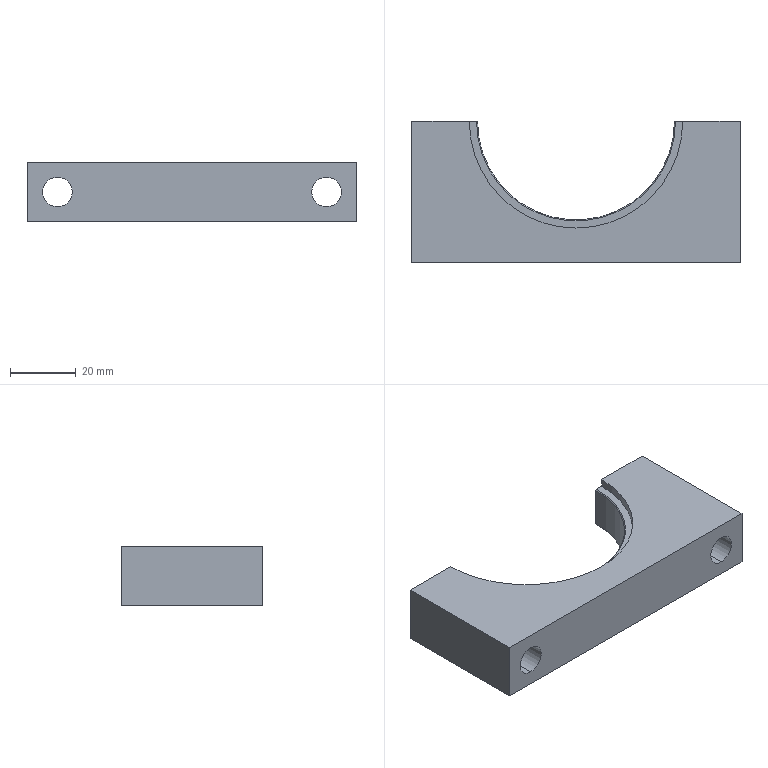Part | SolidWorks | features HoleWzd 2, ICE 2, Chamfer 1, Extrusion 1 | 1 solid | 21 faces | box 100 x 43 x 18 mm | volume 45196 mm3 | plane 10 | cylinder 9 | cone 2 | commonest cylinder face diameters 9 x4 4 x2 65 x2 60 x1
STEP:
#1=CARTESIAN_POINT('',(0.,-34.,7.));
#2=VERTEX_POINT('',#1);
#3=CARTESIAN_POINT('',(0.,-34.,11.));
#4=VERTEX_POINT('',#3);
#5=CARTESIAN_POINT('',(0.,-34.,9.));
#6=DIRECTION('',(0.,1.,0.));
#7=DIRECTION('',(0.,0.,1.));
#8=AXIS2_PLACEMENT_3D('',#5,#6,#7);
#9=CIRCLE('',#8,2.);
#10=EDGE_CURVE('',#2,#4,#9,.T.);
#11=ORIENTED_EDGE('',*,*,#10,.F.);
#12=CARTESIAN_POINT('',(0.,-30.,7.));
#13=VERTEX_POINT('',#12);
#14=CARTESIAN_POINT('',(0.,0.,7.));
#15=DIRECTION('',(0.,1.,0.));
#16=VECTOR('',#15,1000.);
#17=LINE('',#14,#16);
#18=EDGE_CURVE('',#2,#13,#17,.T.);
#19=ORIENTED_EDGE('',*,*,#18,.T.);
#20=CARTESIAN_POINT('',(0.,-30.,11.));
#21=VERTEX_POINT('',#20);
#22=CARTESIAN_POINT('',(0.,-30.,11.));
#23=CARTESIAN_POINT('',(-0.1322,-30.,11.));
#24=CARTESIAN_POINT('',(-0.2622,-29.999,10.987));
#25=CARTESIAN_POINT('',(-0.5178,-29.996,10.936));
#26=CARTESIAN_POINT('',(-0.6449,-29.993,10.898));
#27=CARTESIAN_POINT('',(-0.8871,-29.987,10.797));
#28=CARTESIAN_POINT('',(-1.002,-29.983,10.736));
#29=CARTESIAN_POINT('',(-1.219,-29.975,10.591));
#30=CARTESIAN_POINT('',(-1.322,-29.971,10.506));
#31=CARTESIAN_POINT('',(-1.599,-29.958,10.229));
#32=CARTESIAN_POINT('',(-1.748,-29.949,10.006));
#33=CARTESIAN_POINT('',(-1.947,-29.937,9.525));
#34=CARTESIAN_POINT('',(-2.,-29.933,9.262));
#35=CARTESIAN_POINT('',(-2.,-29.933,8.87));
#36=CARTESIAN_POINT('',(-1.987,-29.934,8.738));
#37=CARTESIAN_POINT('',(-1.936,-29.937,8.481));
#38=CARTESIAN_POINT('',(-1.898,-29.94,8.356));
#39=CARTESIAN_POINT('',(-1.798,-29.946,8.114));
#40=CARTESIAN_POINT('',(-1.735,-29.95,7.997));
#41=CARTESIAN_POINT('',(-1.591,-29.958,7.78));
#42=CARTESIAN_POINT('',(-1.508,-29.962,7.679));
#43=CARTESIAN_POINT('',(-1.321,-29.971,7.493));
#44=CARTESIAN_POINT('',(-1.22,-29.975,7.41));
#45=CARTESIAN_POINT('',(-1.003,-29.983,7.265));
#46=CARTESIAN_POINT('',(-0.8865,-29.987,7.202));
#47=CARTESIAN_POINT('',(-0.6442,-29.993,7.102));
#48=CARTESIAN_POINT('',(-0.5195,-29.996,7.064));
#49=CARTESIAN_POINT('',(-0.2631,-29.999,7.013));
#50=CARTESIAN_POINT('',(-0.1305,-30.,7.));
#51=CARTESIAN_POINT('',(0.,-30.,7.));
#52=B_SPLINE_CURVE_WITH_KNOTS('',3,(#22,#23,#24,#25,#26,#27,#28,#29,#30,#31,#32,#33,#34,#35,#36,#37,#38,#39,#40,#41,#42,#43,#44,#45,#46,#47,#48,#49,#50,#51),.UNSPECIFIED.,.F.,.F.,(4,2,2,2,2,2,2,2,2,2,2,2,2,2,4),(0.,0.0003909,0.0007818,0.001173,0.001564,0.002345,0.003127,0.003518,0.003909,0.0043,0.004691,0.005082,0.005473,0.005864,0.006255),.UNSPECIFIED.);
#53=EDGE_CURVE('',#21,#13,#52,.T.);
#54=ORIENTED_EDGE('',*,*,#53,.F.);
#55=CARTESIAN_POINT('',(0.,0.,11.));
#56=DIRECTION('',(0.,1.,0.));
#57=VECTOR('',#56,1000.);
#58=LINE('',#55,#57);
#59=EDGE_CURVE('',#4,#21,#58,.T.);
#60=ORIENTED_EDGE('',*,*,#59,.F.);
#61=EDGE_LOOP('',(#11,#19,#54,#60));
#62=FACE_OUTER_BOUND('',#61,.T.);
#63=CARTESIAN_POINT('',(0.,0.,9.));
#64=DIRECTION('',(0.,1.,0.));
#65=DIRECTION('',(0.,0.,1.));
#66=AXIS2_PLACEMENT_3D('',#63,#64,#65);
#67=CYLINDRICAL_SURFACE('',#66,2.);
#68=ADVANCED_FACE('',(#62),#67,.F.);
#69=CARTESIAN_POINT('',(-41.,-43.,4.5));
#70=VERTEX_POINT('',#69);
#71=CARTESIAN_POINT('',(-41.,-43.,13.5));
#72=VERTEX_POINT('',#71);
#73=CARTESIAN_POINT('',(-41.,-43.,9.));
#74=DIRECTION('',(0.,1.,0.));
#75=DIRECTION('',(0.,0.,1.));
#76=AXIS2_PLACEMENT_3D('',#73,#74,#75);
#77=CIRCLE('',#76,4.5);
#78=EDGE_CURVE('',#70,#72,#77,.T.);
#79=ORIENTED_EDGE('',*,*,#78,.F.);
#80=CARTESIAN_POINT('',(-41.,0.,4.5));
#81=VERTEX_POINT('',#80);
#82=CARTESIAN_POINT('',(-41.,0.,4.5));
#83=DIRECTION('',(0.,1.,0.));
#84=VECTOR('',#83,1000.);
#85=LINE('',#82,#84);
#86=EDGE_CURVE('',#70,#81,#85,.T.);
#87=ORIENTED_EDGE('',*,*,#86,.T.);
#88=CARTESIAN_POINT('',(-41.,0.,13.5));
#89=VERTEX_POINT('',#88);
#90=CARTESIAN_POINT('',(-41.,0.,9.));
#91=DIRECTION('',(0.,1.,0.));
#92=DIRECTION('',(0.,0.,1.));
#93=AXIS2_PLACEMENT_3D('',#90,#91,#92);
#94=CIRCLE('',#93,4.5);
#95=EDGE_CURVE('',#81,#89,#94,.T.);
#96=ORIENTED_EDGE('',*,*,#95,.T.);
#97=CARTESIAN_POINT('',(-41.,0.,13.5));
#98=DIRECTION('',(0.,1.,0.));
#99=VECTOR('',#98,1000.);
#100=LINE('',#97,#99);
#101=EDGE_CURVE('',#72,#89,#100,.T.);
#102=ORIENTED_EDGE('',*,*,#101,.F.);
#103=EDGE_LOOP('',(#79,#87,#96,#102));
#104=FACE_OUTER_BOUND('',#103,.T.);
#105=CARTESIAN_POINT('',(-41.,0.,9.));
#106=DIRECTION('',(0.,1.,0.));
#107=DIRECTION('',(0.,0.,1.));
#108=AXIS2_PLACEMENT_3D('',#105,#106,#107);
#109=CYLINDRICAL_SURFACE('',#108,4.5);
#110=ADVANCED_FACE('',(#104),#109,.F.);
#111=CARTESIAN_POINT('',(41.,-43.,4.5));
#112=VERTEX_POINT('',#111);
#113=CARTESIAN_POINT('',(41.,-43.,13.5));
#114=VERTEX_POINT('',#113);
#115=CARTESIAN_POINT('',(41.,-43.,9.));
#116=DIRECTION('',(0.,1.,0.));
#117=DIRECTION('',(0.,0.,1.));
#118=AXIS2_PLACEMENT_3D('',#115,#116,#117);
#119=CIRCLE('',#118,4.5);
#120=EDGE_CURVE('',#112,#114,#119,.T.);
#121=ORIENTED_EDGE('',*,*,#120,.F.);
#122=CARTESIAN_POINT('',(41.,0.,4.5));
#123=VERTEX_POINT('',#122);
#124=CARTESIAN_POINT('',(41.,0.,4.5));
#125=DIRECTION('',(0.,1.,0.));
#126=VECTOR('',#125,1000.);
#127=LINE('',#124,#126);
#128=EDGE_CURVE('',#112,#123,#127,.T.);
#129=ORIENTED_EDGE('',*,*,#128,.T.);
#130=CARTESIAN_POINT('',(41.,0.,13.5));
#131=VERTEX_POINT('',#130);
#132=CARTESIAN_POINT('',(41.,0.,9.));
#133=DIRECTION('',(0.,1.,0.));
#134=DIRECTION('',(0.,0.,1.));
#135=AXIS2_PLACEMENT_3D('',#132,#133,#134);
#136=CIRCLE('',#135,4.5);
#137=EDGE_CURVE('',#123,#131,#136,.T.);
#138=ORIENTED_EDGE('',*,*,#137,.T.);
#139=CARTESIAN_POINT('',(41.,0.,13.5));
#140=DIRECTION('',(0.,1.,0.));
#141=VECTOR('',#140,1000.);
#142=LINE('',#139,#141);
#143=EDGE_CURVE('',#114,#131,#142,.T.);
#144=ORIENTED_EDGE('',*,*,#143,.F.);
#145=EDGE_LOOP('',(#121,#129,#138,#144));
#146=FACE_OUTER_BOUND('',#145,.T.);
#147=CARTESIAN_POINT('',(41.,0.,9.));
#148=DIRECTION('',(0.,1.,0.));
#149=DIRECTION('',(0.,0.,1.));
#150=AXIS2_PLACEMENT_3D('',#147,#148,#149);
#151=CYLINDRICAL_SURFACE('',#150,4.5);
#152=ADVANCED_FACE('',(#146),#151,.F.);
#153=ORIENTED_EDGE('',*,*,#53,.T.);
#154=CARTESIAN_POINT('',(0.,-30.,7.));
#155=CARTESIAN_POINT('',(0.261,-30.,7.));
#156=CARTESIAN_POINT('',(0.5242,-29.996,7.052));
#157=CARTESIAN_POINT('',(1.006,-29.984,7.252));
#158=CARTESIAN_POINT('',(1.229,-29.975,7.401));
#159=CARTESIAN_POINT('',(1.505,-29.962,7.677));
#160=CARTESIAN_POINT('',(1.59,-29.958,7.78));
#161=CARTESIAN_POINT('',(1.735,-29.95,7.997));
#162=CARTESIAN_POINT('',(1.797,-29.946,8.112));
#163=CARTESIAN_POINT('',(1.897,-29.94,8.354));
#164=CARTESIAN_POINT('',(1.936,-29.937,8.481));
#165=CARTESIAN_POINT('',(1.987,-29.934,8.737));
#166=CARTESIAN_POINT('',(2.,-29.933,8.866));
#167=CARTESIAN_POINT('',(2.,-29.933,9.13));
#168=CARTESIAN_POINT('',(1.987,-29.934,9.261));
#169=CARTESIAN_POINT('',(1.937,-29.937,9.516));
#170=CARTESIAN_POINT('',(1.898,-29.94,9.643));
#171=CARTESIAN_POINT('',(1.798,-29.946,9.886));
#172=CARTESIAN_POINT('',(1.737,-29.95,10.001));
#173=CARTESIAN_POINT('',(1.592,-29.958,10.218));
#174=CARTESIAN_POINT('',(1.507,-29.962,10.321));
#175=CARTESIAN_POINT('',(1.323,-29.971,10.506));
#176=CARTESIAN_POINT('',(1.222,-29.975,10.588));
#177=CARTESIAN_POINT('',(1.004,-29.983,10.735));
#178=CARTESIAN_POINT('',(0.8877,-29.987,10.797));
#179=CARTESIAN_POINT('',(0.5269,-29.996,10.947));
#180=CARTESIAN_POINT('',(0.2643,-30.,11.));
#181=CARTESIAN_POINT('',(0.,-30.,11.));
#182=B_SPLINE_CURVE_WITH_KNOTS('',3,(#154,#155,#156,#157,#158,#159,#160,#161,#162,#163,#164,#165,#166,#167,#168,#169,#170,#171,#172,#173,#174,#175,#176,#177,#178,#179,#180,#181),.UNSPECIFIED.,.F.,.F.,(4,2,2,2,2,2,2,2,2,2,2,2,2,4),(0.006255,0.007036,0.007818,0.008209,0.0086,0.00899,0.009381,0.009772,0.01016,0.01055,0.01094,0.01134,0.01173,0.01251),.UNSPECIFIED.);
#183=EDGE_CURVE('',#13,#21,#182,.T.);
#184=ORIENTED_EDGE('',*,*,#183,.T.);
#185=EDGE_LOOP('',(#153,#184));
#186=FACE_BOUND('',#185,.T.);
#187=CARTESIAN_POINT('',(30.,0.,15.2));
#188=VERTEX_POINT('',#187);
#189=CARTESIAN_POINT('',(30.,0.,2.8));
#190=VERTEX_POINT('',#189);
#191=CARTESIAN_POINT('',(30.,0.,18.));
#192=DIRECTION('',(0.,0.,-1.));
#193=VECTOR('',#192,1000.);
#194=LINE('',#191,#193);
#195=EDGE_CURVE('',#188,#190,#194,.T.);
#196=ORIENTED_EDGE('',*,*,#195,.T.);
#197=CARTESIAN_POINT('',(-30.,0.,2.8));
#198=VERTEX_POINT('',#197);
#199=CARTESIAN_POINT('',(0.,0.,2.8));
#200=DIRECTION('',(0.,0.,-1.));
#201=DIRECTION('',(-1.,0.,0.));
#202=AXIS2_PLACEMENT_3D('',#199,#200,#201);
#203=CIRCLE('',#202,30.);
#204=EDGE_CURVE('',#190,#198,#203,.T.);
#205=ORIENTED_EDGE('',*,*,#204,.T.);
#206=CARTESIAN_POINT('',(-30.,0.,15.2));
#207=VERTEX_POINT('',#206);
#208=CARTESIAN_POINT('',(-30.,0.,18.));
#209=DIRECTION('',(0.,0.,-1.));
#210=VECTOR('',#209,1000.);
#211=LINE('',#208,#210);
#212=EDGE_CURVE('',#207,#198,#211,.T.);
#213=ORIENTED_EDGE('',*,*,#212,.F.);
#214=CARTESIAN_POINT('',(0.,0.,15.2));
#215=DIRECTION('',(0.,0.,1.));
#216=DIRECTION('',(1.,0.,0.));
#217=AXIS2_PLACEMENT_3D('',#214,#215,#216);
#218=CIRCLE('',#217,30.);
#219=EDGE_CURVE('',#207,#188,#218,.T.);
#220=ORIENTED_EDGE('',*,*,#219,.T.);
#221=EDGE_LOOP('',(#196,#205,#213,#220));
#222=FACE_OUTER_BOUND('',#221,.T.);
#223=CARTESIAN_POINT('',(0.,0.,18.));
#224=DIRECTION('',(0.,0.,-1.));
#225=DIRECTION('',(-1.,0.,0.));
#226=AXIS2_PLACEMENT_3D('',#223,#224,#225);
#227=CYLINDRICAL_SURFACE('',#226,30.);
#228=ADVANCED_FACE('',(#186,#222),#227,.F.);
#229=CARTESIAN_POINT('',(-41.,0.,9.));
#230=DIRECTION('',(0.,1.,0.));
#231=DIRECTION('',(0.,0.,1.));
#232=AXIS2_PLACEMENT_3D('',#229,#230,#231);
#233=CIRCLE('',#232,4.5);
#234=EDGE_CURVE('',#89,#81,#233,.T.);
#235=ORIENTED_EDGE('',*,*,#234,.F.);
#236=ORIENTED_EDGE('',*,*,#95,.F.);
#237=EDGE_LOOP('',(#235,#236));
#238=FACE_BOUND('',#237,.T.);
#239=ORIENTED_EDGE('',*,*,#212,.T.);
#240=CARTESIAN_POINT('',(-30.3,0.,2.5));
#241=VERTEX_POINT('',#240);
#242=CARTESIAN_POINT('',(0.,0.,32.8));
#243=DIRECTION('',(-0.7071,0.,-0.7071));
#244=VECTOR('',#243,1000.);
#245=LINE('',#242,#244);
#246=EDGE_CURVE('',#198,#241,#245,.T.);
#247=ORIENTED_EDGE('',*,*,#246,.T.);
#248=CARTESIAN_POINT('',(-32.5,0.,2.5));
#249=VERTEX_POINT('',#248);
#250=CARTESIAN_POINT('',(-50.,0.,2.5));
#251=DIRECTION('',(1.,0.,0.));
#252=VECTOR('',#251,1000.);
#253=LINE('',#250,#252);
#254=EDGE_CURVE('',#249,#241,#253,.T.);
#255=ORIENTED_EDGE('',*,*,#254,.F.);
#256=CARTESIAN_POINT('',(-32.5,0.,0.));
#257=VERTEX_POINT('',#256);
#258=CARTESIAN_POINT('',(-32.5,0.,2.5));
#259=DIRECTION('',(0.,0.,-1.));
#260=VECTOR('',#259,1000.);
#261=LINE('',#258,#260);
#262=EDGE_CURVE('',#249,#257,#261,.T.);
#263=ORIENTED_EDGE('',*,*,#262,.T.);
#264=CARTESIAN_POINT('',(-50.,0.,0.));
#265=VERTEX_POINT('',#264);
#266=CARTESIAN_POINT('',(-50.,0.,0.));
#267=DIRECTION('',(-1.,0.,0.));
#268=VECTOR('',#267,1000.);
#269=LINE('',#266,#268);
#270=EDGE_CURVE('',#257,#265,#269,.T.);
#271=ORIENTED_EDGE('',*,*,#270,.T.);
#272=CARTESIAN_POINT('',(-50.,0.,18.));
#273=VERTEX_POINT('',#272);
#274=CARTESIAN_POINT('',(-50.,0.,18.));
#275=DIRECTION('',(0.,0.,-1.));
#276=VECTOR('',#275,1000.);
#277=LINE('',#274,#276);
#278=EDGE_CURVE('',#273,#265,#277,.T.);
#279=ORIENTED_EDGE('',*,*,#278,.F.);
#280=CARTESIAN_POINT('',(-32.5,0.,18.));
#281=VERTEX_POINT('',#280);
#282=CARTESIAN_POINT('',(-50.,0.,18.));
#283=DIRECTION('',(-1.,0.,0.));
#284=VECTOR('',#283,1000.);
#285=LINE('',#282,#284);
#286=EDGE_CURVE('',#281,#273,#285,.T.);
#287=ORIENTED_EDGE('',*,*,#286,.F.);
#288=CARTESIAN_POINT('',(-32.5,0.,15.5));
#289=VERTEX_POINT('',#288);
#290=CARTESIAN_POINT('',(-32.5,0.,15.5));
#291=DIRECTION('',(0.,0.,-1.));
#292=VECTOR('',#291,1000.);
#293=LINE('',#290,#292);
#294=EDGE_CURVE('',#281,#289,#293,.T.);
#295=ORIENTED_EDGE('',*,*,#294,.T.);
#296=CARTESIAN_POINT('',(-30.3,0.,15.5));
#297=VERTEX_POINT('',#296);
#298=CARTESIAN_POINT('',(-50.,0.,15.5));
#299=DIRECTION('',(-1.,0.,0.));
#300=VECTOR('',#299,1000.);
#301=LINE('',#298,#300);
#302=EDGE_CURVE('',#297,#289,#301,.T.);
#303=ORIENTED_EDGE('',*,*,#302,.F.);
#304=CARTESIAN_POINT('',(0.,0.,-14.8));
#305=DIRECTION('',(0.7071,0.,-0.7071));
#306=VECTOR('',#305,1000.);
#307=LINE('',#304,#306);
#308=EDGE_CURVE('',#297,#207,#307,.T.);
#309=ORIENTED_EDGE('',*,*,#308,.T.);
#310=EDGE_LOOP('',(#239,#247,#255,#263,#271,#279,#287,#295,#303,#309));
#311=FACE_OUTER_BOUND('',#310,.T.);
#312=CARTESIAN_POINT('',(-50.,0.,18.));
#313=DIRECTION('',(0.,-1.,0.));
#314=DIRECTION('',(1.,0.,0.));
#315=AXIS2_PLACEMENT_3D('',#312,#313,#314);
#316=PLANE('',#315);
#317=ADVANCED_FACE('',(#238,#311),#316,.F.);
#318=CARTESIAN_POINT('',(-50.,-43.,0.));
#319=VERTEX_POINT('',#318);
#320=CARTESIAN_POINT('',(-50.,-43.,0.));
#321=DIRECTION('',(0.,-1.,0.));
#322=VECTOR('',#321,1000.);
#323=LINE('',#320,#322);
#324=EDGE_CURVE('',#265,#319,#323,.T.);
#325=ORIENTED_EDGE('',*,*,#324,.T.);
#326=CARTESIAN_POINT('',(-50.,-43.,18.));
#327=VERTEX_POINT('',#326);
#328=CARTESIAN_POINT('',(-50.,-43.,18.));
#329=DIRECTION('',(0.,0.,-1.));
#330=VECTOR('',#329,1000.);
#331=LINE('',#328,#330);
#332=EDGE_CURVE('',#327,#319,#331,.T.);
#333=ORIENTED_EDGE('',*,*,#332,.F.);
#334=CARTESIAN_POINT('',(-50.,-43.,18.));
#335=DIRECTION('',(0.,-1.,0.));
#336=VECTOR('',#335,1000.);
#337=LINE('',#334,#336);
#338=EDGE_CURVE('',#273,#327,#337,.T.);
#339=ORIENTED_EDGE('',*,*,#338,.F.);
#340=ORIENTED_EDGE('',*,*,#278,.T.);
#341=EDGE_LOOP('',(#325,#333,#339,#340));
#342=FACE_OUTER_BOUND('',#341,.T.);
#343=CARTESIAN_POINT('',(-50.,-43.,18.));
#344=DIRECTION('',(1.,0.,0.));
#345=DIRECTION('',(0.,0.,-1.));
#346=AXIS2_PLACEMENT_3D('',#343,#344,#345);
#347=PLANE('',#346);
#348=ADVANCED_FACE('',(#342),#347,.F.);
#349=CARTESIAN_POINT('',(-41.,-43.,9.));
#350=DIRECTION('',(0.,1.,0.));
#351=DIRECTION('',(0.,0.,1.));
#352=AXIS2_PLACEMENT_3D('',#349,#350,#351);
#353=CIRCLE('',#352,4.5);
#354=EDGE_CURVE('',#72,#70,#353,.T.);
#355=ORIENTED_EDGE('',*,*,#354,.T.);
#356=ORIENTED_EDGE('',*,*,#78,.T.);
#357=EDGE_LOOP('',(#355,#356));
#358=FACE_BOUND('',#357,.T.);
#359=CARTESIAN_POINT('',(41.,-43.,9.));
#360=DIRECTION('',(0.,1.,0.));
#361=DIRECTION('',(0.,0.,1.));
#362=AXIS2_PLACEMENT_3D('',#359,#360,#361);
#363=CIRCLE('',#362,4.5);
#364=EDGE_CURVE('',#114,#112,#363,.T.);
#365=ORIENTED_EDGE('',*,*,#364,.T.);
#366=ORIENTED_EDGE('',*,*,#120,.T.);
#367=EDGE_LOOP('',(#365,#366));
#368=FACE_BOUND('',#367,.T.);
#369=CARTESIAN_POINT('',(50.,-43.,0.));
#370=VERTEX_POINT('',#369);
#371=CARTESIAN_POINT('',(-50.,-43.,0.));
#372=DIRECTION('',(1.,0.,0.));
#373=VECTOR('',#372,1000.);
#374=LINE('',#371,#373);
#375=EDGE_CURVE('',#319,#370,#374,.T.);
#376=ORIENTED_EDGE('',*,*,#375,.T.);
#377=CARTESIAN_POINT('',(50.,-43.,18.));
#378=VERTEX_POINT('',#377);
#379=CARTESIAN_POINT('',(50.,-43.,18.));
#380=DIRECTION('',(0.,0.,-1.));
#381=VECTOR('',#380,1000.);
#382=LINE('',#379,#381);
#383=EDGE_CURVE('',#378,#370,#382,.T.);
#384=ORIENTED_EDGE('',*,*,#383,.F.);
#385=CARTESIAN_POINT('',(-50.,-43.,18.));
#386=DIRECTION('',(1.,0.,0.));
#387=VECTOR('',#386,1000.);
#388=LINE('',#385,#387);
#389=EDGE_CURVE('',#327,#378,#388,.T.);
#390=ORIENTED_EDGE('',*,*,#389,.F.);
#391=ORIENTED_EDGE('',*,*,#332,.T.);
#392=EDGE_LOOP('',(#376,#384,#390,#391));
#393=FACE_OUTER_BOUND('',#392,.T.);
#394=CARTESIAN_POINT('',(-50.,-43.,18.));
#395=DIRECTION('',(0.,1.,0.));
#396=DIRECTION('',(-1.,0.,0.));
#397=AXIS2_PLACEMENT_3D('',#394,#395,#396);
#398=PLANE('',#397);
#399=ADVANCED_FACE('',(#358,#368,#393),#398,.F.);
#400=CARTESIAN_POINT('',(50.,0.,0.));
#401=VERTEX_POINT('',#400);
#402=CARTESIAN_POINT('',(50.,-43.,0.));
#403=DIRECTION('',(0.,1.,0.));
#404=VECTOR('',#403,1000.);
#405=LINE('',#402,#404);
#406=EDGE_CURVE('',#370,#401,#405,.T.);
#407=ORIENTED_EDGE('',*,*,#406,.T.);
#408=CARTESIAN_POINT('',(50.,0.,18.));
#409=VERTEX_POINT('',#408);
#410=CARTESIAN_POINT('',(50.,0.,18.));
#411=DIRECTION('',(0.,0.,-1.));
#412=VECTOR('',#411,1000.);
#413=LINE('',#410,#412);
#414=EDGE_CURVE('',#409,#401,#413,.T.);
#415=ORIENTED_EDGE('',*,*,#414,.F.);
#416=CARTESIAN_POINT('',(50.,-43.,18.));
#417=DIRECTION('',(0.,1.,0.));
#418=VECTOR('',#417,1000.);
#419=LINE('',#416,#418);
#420=EDGE_CURVE('',#378,#409,#419,.T.);
#421=ORIENTED_EDGE('',*,*,#420,.F.);
#422=ORIENTED_EDGE('',*,*,#383,.T.);
#423=EDGE_LOOP('',(#407,#415,#421,#422));
#424=FACE_OUTER_BOUND('',#423,.T.);
#425=CARTESIAN_POINT('',(50.,-43.,18.));
#426=DIRECTION('',(-1.,0.,0.));
#427=DIRECTION('',(0.,-1.,0.));
#428=AXIS2_PLACEMENT_3D('',#425,#426,#427);
#429=PLANE('',#428);
#430=ADVANCED_FACE('',(#424),#429,.F.);
#431=CARTESIAN_POINT('',(41.,0.,9.));
#432=DIRECTION('',(0.,1.,0.));
#433=DIRECTION('',(0.,0.,1.));
#434=AXIS2_PLACEMENT_3D('',#431,#432,#433);
#435=CIRCLE('',#434,4.5);
#436=EDGE_CURVE('',#131,#123,#435,.T.);
#437=ORIENTED_EDGE('',*,*,#436,.F.);
#438=ORIENTED_EDGE('',*,*,#137,.F.);
#439=EDGE_LOOP('',(#437,#438));
#440=FACE_BOUND('',#439,.T.);
#441=CARTESIAN_POINT('',(30.3,0.,2.5));
#442=VERTEX_POINT('',#441);
#443=CARTESIAN_POINT('',(32.5,0.,2.5));
#444=VERTEX_POINT('',#443);
#445=CARTESIAN_POINT('',(30.,0.,2.5));
#446=DIRECTION('',(1.,0.,0.));
#447=VECTOR('',#446,1000.);
#448=LINE('',#445,#447);
#449=EDGE_CURVE('',#442,#444,#448,.T.);
#450=ORIENTED_EDGE('',*,*,#449,.F.);
#451=CARTESIAN_POINT('',(0.,0.,32.8));
#452=DIRECTION('',(-0.7071,0.,0.7071));
#453=VECTOR('',#452,1000.);
#454=LINE('',#451,#453);
#455=EDGE_CURVE('',#442,#190,#454,.T.);
#456=ORIENTED_EDGE('',*,*,#455,.T.);
#457=ORIENTED_EDGE('',*,*,#195,.F.);
#458=CARTESIAN_POINT('',(30.3,0.,15.5));
#459=VERTEX_POINT('',#458);
#460=CARTESIAN_POINT('',(0.,0.,-14.8));
#461=DIRECTION('',(0.7071,0.,0.7071));
#462=VECTOR('',#461,1000.);
#463=LINE('',#460,#462);
#464=EDGE_CURVE('',#188,#459,#463,.T.);
#465=ORIENTED_EDGE('',*,*,#464,.T.);
#466=CARTESIAN_POINT('',(32.5,0.,15.5));
#467=VERTEX_POINT('',#466);
#468=CARTESIAN_POINT('',(30.,0.,15.5));
#469=DIRECTION('',(-1.,0.,0.));
#470=VECTOR('',#469,1000.);
#471=LINE('',#468,#470);
#472=EDGE_CURVE('',#467,#459,#471,.T.);
#473=ORIENTED_EDGE('',*,*,#472,.F.);
#474=CARTESIAN_POINT('',(32.5,0.,18.));
#475=VERTEX_POINT('',#474);
#476=CARTESIAN_POINT('',(32.5,0.,15.5));
#477=DIRECTION('',(0.,0.,1.));
#478=VECTOR('',#477,1000.);
#479=LINE('',#476,#478);
#480=EDGE_CURVE('',#467,#475,#479,.T.);
#481=ORIENTED_EDGE('',*,*,#480,.T.);
#482=CARTESIAN_POINT('',(30.,0.,18.));
#483=DIRECTION('',(-1.,0.,0.));
#484=VECTOR('',#483,1000.);
#485=LINE('',#482,#484);
#486=EDGE_CURVE('',#409,#475,#485,.T.);
#487=ORIENTED_EDGE('',*,*,#486,.F.);
#488=ORIENTED_EDGE('',*,*,#414,.T.);
#489=CARTESIAN_POINT('',(32.5,0.,0.));
#490=VERTEX_POINT('',#489);
#491=CARTESIAN_POINT('',(30.,0.,0.));
#492=DIRECTION('',(-1.,0.,0.));
#493=VECTOR('',#492,1000.);
#494=LINE('',#491,#493);
#495=EDGE_CURVE('',#401,#490,#494,.T.);
#496=ORIENTED_EDGE('',*,*,#495,.T.);
#497=CARTESIAN_POINT('',(32.5,0.,2.5));
#498=DIRECTION('',(0.,0.,1.));
#499=VECTOR('',#498,1000.);
#500=LINE('',#497,#499);
#501=EDGE_CURVE('',#490,#444,#500,.T.);
#502=ORIENTED_EDGE('',*,*,#501,.T.);
#503=EDGE_LOOP('',(#450,#456,#457,#465,#473,#481,#487,#488,#496,#502));
#504=FACE_OUTER_BOUND('',#503,.T.);
#505=CARTESIAN_POINT('',(30.,0.,18.));
#506=DIRECTION('',(0.,-1.,0.));
#507=DIRECTION('',(1.,0.,0.));
#508=AXIS2_PLACEMENT_3D('',#505,#506,#507);
#509=PLANE('',#508);
#510=ADVANCED_FACE('',(#440,#504),#509,.F.);
#511=CARTESIAN_POINT('',(0.,0.,18.));
#512=DIRECTION('',(0.,0.,1.));
#513=DIRECTION('',(1.,0.,0.));
#514=AXIS2_PLACEMENT_3D('',#511,#512,#513);
#515=CIRCLE('',#514,32.5);
#516=EDGE_CURVE('',#281,#475,#515,.T.);
#517=ORIENTED_EDGE('',*,*,#516,.F.);
#518=ORIENTED_EDGE('',*,*,#286,.T.);
#519=ORIENTED_EDGE('',*,*,#338,.T.);
#520=ORIENTED_EDGE('',*,*,#389,.T.);
#521=ORIENTED_EDGE('',*,*,#420,.T.);
#522=ORIENTED_EDGE('',*,*,#486,.T.);
#523=EDGE_LOOP('',(#517,#518,#519,#520,#521,#522));
#524=FACE_OUTER_BOUND('',#523,.T.);
#525=CARTESIAN_POINT('',(0.,0.,18.));
#526=DIRECTION('',(0.,0.,1.));
#527=DIRECTION('',(1.,0.,0.));
#528=AXIS2_PLACEMENT_3D('',#525,#526,#527);
#529=PLANE('',#528);
#530=ADVANCED_FACE('',(#524),#529,.T.);
#531=ORIENTED_EDGE('',*,*,#270,.F.);
#532=CARTESIAN_POINT('',(0.,0.,0.));
#533=DIRECTION('',(0.,0.,1.));
#534=DIRECTION('',(1.,0.,0.));
#535=AXIS2_PLACEMENT_3D('',#532,#533,#534);
#536=CIRCLE('',#535,32.5);
#537=EDGE_CURVE('',#257,#490,#536,.T.);
#538=ORIENTED_EDGE('',*,*,#537,.T.);
#539=ORIENTED_EDGE('',*,*,#495,.F.);
#540=ORIENTED_EDGE('',*,*,#406,.F.);
#541=ORIENTED_EDGE('',*,*,#375,.F.);
#542=ORIENTED_EDGE('',*,*,#324,.F.);
#543=EDGE_LOOP('',(#531,#538,#539,#540,#541,#542));
#544=FACE_OUTER_BOUND('',#543,.T.);
#545=CARTESIAN_POINT('',(0.,0.,0.));
#546=DIRECTION('',(0.,0.,1.));
#547=DIRECTION('',(1.,0.,0.));
#548=AXIS2_PLACEMENT_3D('',#545,#546,#547);
#549=PLANE('',#548);
#550=ADVANCED_FACE('',(#544),#549,.F.);
#551=ORIENTED_EDGE('',*,*,#472,.T.);
#552=CARTESIAN_POINT('',(0.,0.,15.5));
#553=DIRECTION('',(0.,0.,-1.));
#554=DIRECTION('',(1.,0.,0.));
#555=AXIS2_PLACEMENT_3D('',#552,#553,#554);
#556=CIRCLE('',#555,30.3);
#557=EDGE_CURVE('',#459,#297,#556,.T.);
#558=ORIENTED_EDGE('',*,*,#557,.T.);
#559=ORIENTED_EDGE('',*,*,#302,.T.);
#560=CARTESIAN_POINT('',(0.,0.,15.5));
#561=DIRECTION('',(0.,0.,1.));
#562=DIRECTION('',(1.,0.,0.));
#563=AXIS2_PLACEMENT_3D('',#560,#561,#562);
#564=CIRCLE('',#563,32.5);
#565=EDGE_CURVE('',#289,#467,#564,.T.);
#566=ORIENTED_EDGE('',*,*,#565,.T.);
#567=EDGE_LOOP('',(#551,#558,#559,#566));
#568=FACE_OUTER_BOUND('',#567,.T.);
#569=CARTESIAN_POINT('',(0.,0.,15.5));
#570=DIRECTION('',(0.,0.,1.));
#571=DIRECTION('',(1.,0.,0.));
#572=AXIS2_PLACEMENT_3D('',#569,#570,#571);
#573=PLANE('',#572);
#574=ADVANCED_FACE('',(#568),#573,.T.);
#575=ORIENTED_EDGE('',*,*,#516,.T.);
#576=ORIENTED_EDGE('',*,*,#480,.F.);
#577=ORIENTED_EDGE('',*,*,#565,.F.);
#578=ORIENTED_EDGE('',*,*,#294,.F.);
#579=EDGE_LOOP('',(#575,#576,#577,#578));
#580=FACE_OUTER_BOUND('',#579,.T.);
#581=CARTESIAN_POINT('',(0.,0.,15.5));
#582=DIRECTION('',(0.,0.,1.));
#583=DIRECTION('',(1.,0.,0.));
#584=AXIS2_PLACEMENT_3D('',#581,#582,#583);
#585=CYLINDRICAL_SURFACE('',#584,32.5);
#586=ADVANCED_FACE('',(#580),#585,.F.);
#587=ORIENTED_EDGE('',*,*,#254,.T.);
#588=CARTESIAN_POINT('',(0.,0.,2.5));
#589=DIRECTION('',(0.,0.,1.));
#590=DIRECTION('',(-1.,0.,0.));
#591=AXIS2_PLACEMENT_3D('',#588,#589,#590);
#592=CIRCLE('',#591,30.3);
#593=EDGE_CURVE('',#241,#442,#592,.T.);
#594=ORIENTED_EDGE('',*,*,#593,.T.);
#595=ORIENTED_EDGE('',*,*,#449,.T.);
#596=CARTESIAN_POINT('',(0.,0.,2.5));
#597=DIRECTION('',(0.,0.,-1.));
#598=DIRECTION('',(-1.,0.,0.));
#599=AXIS2_PLACEMENT_3D('',#596,#597,#598);
#600=CIRCLE('',#599,32.5);
#601=EDGE_CURVE('',#444,#249,#600,.T.);
#602=ORIENTED_EDGE('',*,*,#601,.T.);
#603=EDGE_LOOP('',(#587,#594,#595,#602));
#604=FACE_OUTER_BOUND('',#603,.T.);
#605=CARTESIAN_POINT('',(0.,0.,2.5));
#606=DIRECTION('',(0.,0.,-1.));
#607=DIRECTION('',(-1.,0.,0.));
#608=AXIS2_PLACEMENT_3D('',#605,#606,#607);
#609=PLANE('',#608);
#610=ADVANCED_FACE('',(#604),#609,.T.);
#611=ORIENTED_EDGE('',*,*,#601,.F.);
#612=ORIENTED_EDGE('',*,*,#501,.F.);
#613=ORIENTED_EDGE('',*,*,#537,.F.);
#614=ORIENTED_EDGE('',*,*,#262,.F.);
#615=EDGE_LOOP('',(#611,#612,#613,#614));
#616=FACE_OUTER_BOUND('',#615,.T.);
#617=CARTESIAN_POINT('',(0.,0.,2.5));
#618=DIRECTION('',(0.,0.,-1.));
#619=DIRECTION('',(-1.,0.,0.));
#620=AXIS2_PLACEMENT_3D('',#617,#618,#619);
#621=CYLINDRICAL_SURFACE('',#620,32.5);
#622=ADVANCED_FACE('',(#616),#621,.F.);
#623=ORIENTED_EDGE('',*,*,#246,.F.);
#624=ORIENTED_EDGE('',*,*,#204,.F.);
#625=ORIENTED_EDGE('',*,*,#455,.F.);
#626=ORIENTED_EDGE('',*,*,#593,.F.);
#627=EDGE_LOOP('',(#623,#624,#625,#626));
#628=FACE_OUTER_BOUND('',#627,.T.);
#629=CARTESIAN_POINT('',(0.,0.,2.5));
#630=DIRECTION('',(0.,0.,-1.));
#631=DIRECTION('',(-1.,0.,0.));
#632=AXIS2_PLACEMENT_3D('',#629,#630,#631);
#633=CONICAL_SURFACE('',#632,30.3,0.7854);
#634=ADVANCED_FACE('',(#628),#633,.F.);
#635=ORIENTED_EDGE('',*,*,#464,.F.);
#636=ORIENTED_EDGE('',*,*,#219,.F.);
#637=ORIENTED_EDGE('',*,*,#308,.F.);
#638=ORIENTED_EDGE('',*,*,#557,.F.);
#639=EDGE_LOOP('',(#635,#636,#637,#638));
#640=FACE_OUTER_BOUND('',#639,.T.);
#641=CARTESIAN_POINT('',(0.,0.,15.5));
#642=DIRECTION('',(0.,0.,1.));
#643=DIRECTION('',(1.,0.,0.));
#644=AXIS2_PLACEMENT_3D('',#641,#642,#643);
#645=CONICAL_SURFACE('',#644,30.3,0.7854);
#646=ADVANCED_FACE('',(#640),#645,.F.);
#647=ORIENTED_EDGE('',*,*,#128,.F.);
#648=ORIENTED_EDGE('',*,*,#364,.F.);
#649=ORIENTED_EDGE('',*,*,#143,.T.);
#650=ORIENTED_EDGE('',*,*,#436,.T.);
#651=EDGE_LOOP('',(#647,#648,#649,#650));
#652=FACE_OUTER_BOUND('',#651,.T.);
#653=CARTESIAN_POINT('',(41.,0.,9.));
#654=DIRECTION('',(0.,1.,0.));
#655=DIRECTION('',(0.,0.,1.));
#656=AXIS2_PLACEMENT_3D('',#653,#654,#655);
#657=CYLINDRICAL_SURFACE('',#656,4.5);
#658=ADVANCED_FACE('',(#652),#657,.F.);
#659=ORIENTED_EDGE('',*,*,#86,.F.);
#660=ORIENTED_EDGE('',*,*,#354,.F.);
#661=ORIENTED_EDGE('',*,*,#101,.T.);
#662=ORIENTED_EDGE('',*,*,#234,.T.);
#663=EDGE_LOOP('',(#659,#660,#661,#662));
#664=FACE_OUTER_BOUND('',#663,.T.);
#665=CARTESIAN_POINT('',(-41.,0.,9.));
#666=DIRECTION('',(0.,1.,0.));
#667=DIRECTION('',(0.,0.,1.));
#668=AXIS2_PLACEMENT_3D('',#665,#666,#667);
#669=CYLINDRICAL_SURFACE('',#668,4.5);
#670=ADVANCED_FACE('',(#664),#669,.F.);
#671=ORIENTED_EDGE('',*,*,#18,.F.);
#672=CARTESIAN_POINT('',(0.,-34.,9.));
#673=DIRECTION('',(0.,1.,0.));
#674=DIRECTION('',(0.,0.,1.));
#675=AXIS2_PLACEMENT_3D('',#672,#673,#674);
#676=CIRCLE('',#675,2.);
#677=EDGE_CURVE('',#4,#2,#676,.T.);
#678=ORIENTED_EDGE('',*,*,#677,.F.);
#679=ORIENTED_EDGE('',*,*,#59,.T.);
#680=ORIENTED_EDGE('',*,*,#183,.F.);
#681=EDGE_LOOP('',(#671,#678,#679,#680));
#682=FACE_OUTER_BOUND('',#681,.T.);
#683=CARTESIAN_POINT('',(0.,0.,9.));
#684=DIRECTION('',(0.,1.,0.));
#685=DIRECTION('',(0.,0.,1.));
#686=AXIS2_PLACEMENT_3D('',#683,#684,#685);
#687=CYLINDRICAL_SURFACE('',#686,2.);
#688=ADVANCED_FACE('',(#682),#687,.F.);
#689=ORIENTED_EDGE('',*,*,#677,.T.);
#690=ORIENTED_EDGE('',*,*,#10,.T.);
#691=EDGE_LOOP('',(#689,#690));
#692=FACE_OUTER_BOUND('',#691,.T.);
#693=CARTESIAN_POINT('',(0.,-34.,9.));
#694=DIRECTION('',(0.,-1.,0.));
#695=DIRECTION('',(0.,0.,-1.));
#696=AXIS2_PLACEMENT_3D('',#693,#694,#695);
#697=PLANE('',#696);
#698=ADVANCED_FACE('',(#692),#697,.F.);
#699=CLOSED_SHELL('',(#68,#110,#152,#228,#317,#348,#399,#430,#510,#530,#550,#574,#586,#610,#622,#634,#646,#658,#670,#688,#698));
#700=MANIFOLD_SOLID_BREP('',#699);
#701=CARTESIAN_POINT('',(0.,0.,0.));
#702=DIRECTION('',(0.,0.,1.));
#703=DIRECTION('',(1.,0.,0.));
#704=AXIS2_PLACEMENT_3D('',#701,#702,#703);
#705=(LENGTH_UNIT()NAMED_UNIT(*)SI_UNIT(.MILLI.,.METRE.));
#706=UNCERTAINTY_MEASURE_WITH_UNIT(LENGTH_MEASURE(0.00001),#705,'','');
#707=(NAMED_UNIT(*)PLANE_ANGLE_UNIT()SI_UNIT($,.RADIAN.));
#708=(NAMED_UNIT(*)SI_UNIT($,.STERADIAN.)SOLID_ANGLE_UNIT());
#709=(GEOMETRIC_REPRESENTATION_CONTEXT(3)GLOBAL_UNCERTAINTY_ASSIGNED_CONTEXT((#706))GLOBAL_UNIT_ASSIGNED_CONTEXT((#705,#707,#708))REPRESENTATION_CONTEXT('',''));
#710=ADVANCED_BREP_SHAPE_REPRESENTATION('',(#700,#704),#709);